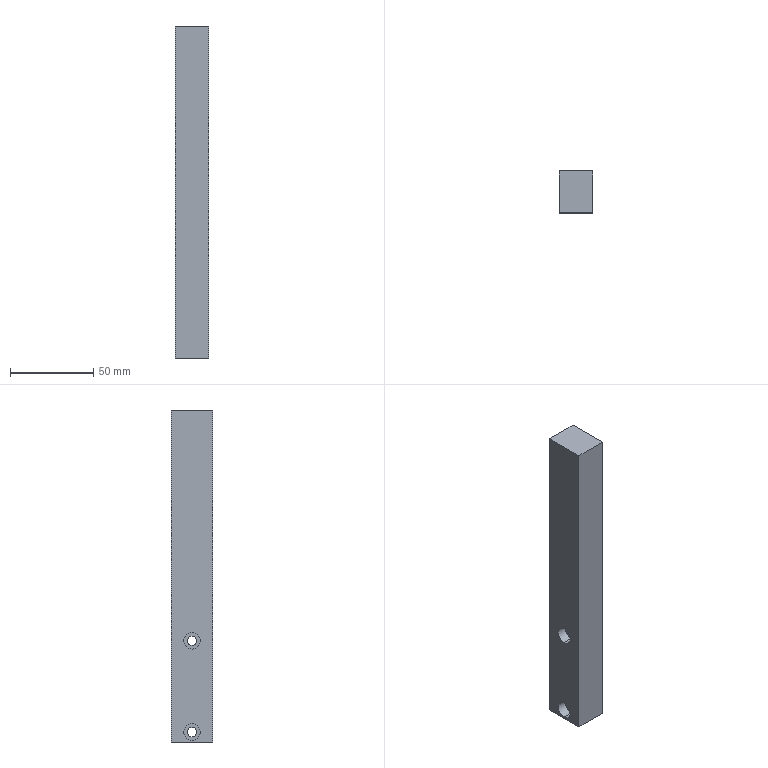Part | STEP file | PN_0058 push block | 1 solid | 16 faces | box 20 x 25 x 200 mm | volume 98425 mm3 | cylinder 8 | plane 8 | commonest cylinder face diameters 5.5 x4 10 x4
STEP:
#1=CARTESIAN_POINT('',(0.,0.,0.));
#2=DIRECTION('',(0.,0.,1.));
#3=DIRECTION('',(1.,0.,0.));
#4=AXIS2_PLACEMENT_3D('',#1,#2,#3);
#5=CARTESIAN_POINT('',(-4.3,0.,11.));
#6=VERTEX_POINT('',#5);
#7=CARTESIAN_POINT('',(-10.,0.,11.));
#8=VERTEX_POINT('',#7);
#9=CARTESIAN_POINT('',(-10.,0.,11.));
#10=DIRECTION('',(-1.,0.,0.));
#11=VECTOR('',#10,1.);
#12=LINE('',#9,#11);
#13=CARTESIAN_POINT('',(-10.,0.,6.));
#14=DIRECTION('',(-1.,0.,0.));
#15=DIRECTION('',(0.,0.,1.));
#16=AXIS2_PLACEMENT_3D('',#13,#14,#15);
#17=CYLINDRICAL_SURFACE('',#16,5.);
#18=CARTESIAN_POINT('',(6.283,0.));
#19=DIRECTION('',(0.,1.));
#20=VECTOR('',#19,1.);
#21=LINE('',#18,#20);
#22=(GEOMETRIC_REPRESENTATION_CONTEXT(2)PARAMETRIC_REPRESENTATION_CONTEXT()REPRESENTATION_CONTEXT('',''));
#23=DEFINITIONAL_REPRESENTATION('',(#21),#22);
#24=PCURVE('',#17,#23);
#25=CARTESIAN_POINT('',(-10.,0.,6.));
#26=DIRECTION('',(-1.,0.,0.));
#27=DIRECTION('',(0.,0.,1.));
#28=AXIS2_PLACEMENT_3D('',#25,#26,#27);
#29=CYLINDRICAL_SURFACE('',#28,5.);
#30=CARTESIAN_POINT('',(0.,0.));
#31=DIRECTION('',(0.,1.));
#32=VECTOR('',#31,1.);
#33=LINE('',#30,#32);
#34=(GEOMETRIC_REPRESENTATION_CONTEXT(2)PARAMETRIC_REPRESENTATION_CONTEXT()REPRESENTATION_CONTEXT('',''));
#35=DEFINITIONAL_REPRESENTATION('',(#33),#34);
#36=PCURVE('',#29,#35);
#37=SURFACE_CURVE('',#12,(#24,#36),.PCURVE_S1.);
#38=EDGE_CURVE('',#6,#8,#37,.T.);
#39=ORIENTED_EDGE('',*,*,#38,.T.);
#40=CARTESIAN_POINT('',(-10.,0.,1.));
#41=VERTEX_POINT('',#40);
#42=CARTESIAN_POINT('',(-10.,0.,6.));
#43=DIRECTION('',(-1.,0.,0.));
#44=DIRECTION('',(0.,0.,1.));
#45=AXIS2_PLACEMENT_3D('',#42,#43,#44);
#46=CIRCLE('',#45,5.);
#47=CARTESIAN_POINT('',(0.,0.));
#48=DIRECTION('',(1.,0.));
#49=VECTOR('',#48,1.);
#50=LINE('',#47,#49);
#51=(GEOMETRIC_REPRESENTATION_CONTEXT(2)PARAMETRIC_REPRESENTATION_CONTEXT()REPRESENTATION_CONTEXT('',''));
#52=DEFINITIONAL_REPRESENTATION('',(#50),#51);
#53=PCURVE('',#17,#52);
#54=CARTESIAN_POINT('',(-10.,12.5,0.));
#55=DIRECTION('',(1.,0.,0.));
#56=DIRECTION('',(0.,0.,-1.));
#57=AXIS2_PLACEMENT_3D('',#54,#55,#56);
#58=PLANE('',#57);
#59=CARTESIAN_POINT('',(-11.,-12.5));
#60=CARTESIAN_POINT('',(-11.,-3.84));
#61=CARTESIAN_POINT('',(-3.5,-8.17));
#62=CARTESIAN_POINT('',(4.,-12.5));
#63=CARTESIAN_POINT('',(-3.5,-16.83));
#64=CARTESIAN_POINT('',(-11.,-21.16));
#65=CARTESIAN_POINT('',(-11.,-12.5));
#66=(BOUNDED_CURVE()B_SPLINE_CURVE(2,(#59,#60,#61,#62,#63,#64,#65),.UNSPECIFIED.,.T.,.F.)B_SPLINE_CURVE_WITH_KNOTS((1,2,2,2,2,1),(-2.094,0.,2.094,4.189,6.283,8.378),.UNSPECIFIED.)CURVE()GEOMETRIC_REPRESENTATION_ITEM()RATIONAL_B_SPLINE_CURVE((1.,0.5,1.,0.5,1.,0.5,1.))REPRESENTATION_ITEM(''));
#67=(GEOMETRIC_REPRESENTATION_CONTEXT(2)PARAMETRIC_REPRESENTATION_CONTEXT()REPRESENTATION_CONTEXT('',''));
#68=DEFINITIONAL_REPRESENTATION('',(#66),#67);
#69=PCURVE('',#58,#68);
#70=SURFACE_CURVE('',#46,(#53,#69),.PCURVE_S1.);
#71=EDGE_CURVE('',#41,#8,#70,.T.);
#72=ORIENTED_EDGE('',*,*,#71,.F.);
#73=CARTESIAN_POINT('',(-4.3,0.,1.));
#74=VERTEX_POINT('',#73);
#75=CARTESIAN_POINT('',(-10.,0.,1.));
#76=DIRECTION('',(-1.,0.,0.));
#77=VECTOR('',#76,1.);
#78=LINE('',#75,#77);
#79=CARTESIAN_POINT('',(3.142,0.));
#80=DIRECTION('',(0.,1.));
#81=VECTOR('',#80,1.);
#82=LINE('',#79,#81);
#83=(GEOMETRIC_REPRESENTATION_CONTEXT(2)PARAMETRIC_REPRESENTATION_CONTEXT()REPRESENTATION_CONTEXT('',''));
#84=DEFINITIONAL_REPRESENTATION('',(#82),#83);
#85=PCURVE('',#17,#84);
#86=CARTESIAN_POINT('',(3.142,0.));
#87=DIRECTION('',(0.,1.));
#88=VECTOR('',#87,1.);
#89=LINE('',#86,#88);
#90=(GEOMETRIC_REPRESENTATION_CONTEXT(2)PARAMETRIC_REPRESENTATION_CONTEXT()REPRESENTATION_CONTEXT('',''));
#91=DEFINITIONAL_REPRESENTATION('',(#89),#90);
#92=PCURVE('',#29,#91);
#93=SURFACE_CURVE('',#78,(#85,#92),.PCURVE_S1.);
#94=EDGE_CURVE('',#74,#41,#93,.T.);
#95=ORIENTED_EDGE('',*,*,#94,.F.);
#96=CARTESIAN_POINT('',(-4.3,0.,6.));
#97=DIRECTION('',(-1.,0.,0.));
#98=DIRECTION('',(0.,0.,1.));
#99=AXIS2_PLACEMENT_3D('',#96,#97,#98);
#100=CIRCLE('',#99,5.);
#101=CARTESIAN_POINT('',(0.,-5.7));
#102=DIRECTION('',(1.,0.));
#103=VECTOR('',#102,1.);
#104=LINE('',#101,#103);
#105=(GEOMETRIC_REPRESENTATION_CONTEXT(2)PARAMETRIC_REPRESENTATION_CONTEXT()REPRESENTATION_CONTEXT('',''));
#106=DEFINITIONAL_REPRESENTATION('',(#104),#105);
#107=PCURVE('',#17,#106);
#108=CARTESIAN_POINT('',(-4.3,2.75,6.));
#109=DIRECTION('',(1.,0.,0.));
#110=DIRECTION('',(0.,0.,-1.));
#111=AXIS2_PLACEMENT_3D('',#108,#109,#110);
#112=PLANE('',#111);
#113=CARTESIAN_POINT('',(-5.,-2.75));
#114=CARTESIAN_POINT('',(-5.,5.91));
#115=CARTESIAN_POINT('',(2.5,1.58));
#116=CARTESIAN_POINT('',(10.,-2.75));
#117=CARTESIAN_POINT('',(2.5,-7.08));
#118=CARTESIAN_POINT('',(-5.,-11.41));
#119=CARTESIAN_POINT('',(-5.,-2.75));
#120=(BOUNDED_CURVE()B_SPLINE_CURVE(2,(#113,#114,#115,#116,#117,#118,#119),.UNSPECIFIED.,.T.,.F.)B_SPLINE_CURVE_WITH_KNOTS((1,2,2,2,2,1),(-2.094,0.,2.094,4.189,6.283,8.378),.UNSPECIFIED.)CURVE()GEOMETRIC_REPRESENTATION_ITEM()RATIONAL_B_SPLINE_CURVE((1.,0.5,1.,0.5,1.,0.5,1.))REPRESENTATION_ITEM(''));
#121=(GEOMETRIC_REPRESENTATION_CONTEXT(2)PARAMETRIC_REPRESENTATION_CONTEXT()REPRESENTATION_CONTEXT('',''));
#122=DEFINITIONAL_REPRESENTATION('',(#120),#121);
#123=PCURVE('',#112,#122);
#124=SURFACE_CURVE('',#100,(#107,#123),.PCURVE_S1.);
#125=EDGE_CURVE('',#74,#6,#124,.T.);
#126=ORIENTED_EDGE('',*,*,#125,.T.);
#127=EDGE_LOOP('',(#39,#72,#95,#126));
#128=FACE_BOUND('',#127,.F.);
#129=ADVANCED_FACE('',(#128),#17,.F.);
#130=CARTESIAN_POINT('',(10.,0.,8.75));
#131=VERTEX_POINT('',#130);
#132=CARTESIAN_POINT('',(-4.3,0.,8.75));
#133=VERTEX_POINT('',#132);
#134=CARTESIAN_POINT('',(-10.,0.,8.75));
#135=DIRECTION('',(-1.,0.,0.));
#136=VECTOR('',#135,1.);
#137=LINE('',#134,#136);
#138=CARTESIAN_POINT('',(-10.,0.,6.));
#139=DIRECTION('',(-1.,0.,0.));
#140=DIRECTION('',(0.,0.,1.));
#141=AXIS2_PLACEMENT_3D('',#138,#139,#140);
#142=CYLINDRICAL_SURFACE('',#141,2.75);
#143=CARTESIAN_POINT('',(6.283,0.));
#144=DIRECTION('',(0.,1.));
#145=VECTOR('',#144,1.);
#146=LINE('',#143,#145);
#147=(GEOMETRIC_REPRESENTATION_CONTEXT(2)PARAMETRIC_REPRESENTATION_CONTEXT()REPRESENTATION_CONTEXT('',''));
#148=DEFINITIONAL_REPRESENTATION('',(#146),#147);
#149=PCURVE('',#142,#148);
#150=CARTESIAN_POINT('',(-10.,0.,6.));
#151=DIRECTION('',(-1.,0.,0.));
#152=DIRECTION('',(0.,0.,1.));
#153=AXIS2_PLACEMENT_3D('',#150,#151,#152);
#154=CYLINDRICAL_SURFACE('',#153,2.75);
#155=CARTESIAN_POINT('',(0.,0.));
#156=DIRECTION('',(0.,1.));
#157=VECTOR('',#156,1.);
#158=LINE('',#155,#157);
#159=(GEOMETRIC_REPRESENTATION_CONTEXT(2)PARAMETRIC_REPRESENTATION_CONTEXT()REPRESENTATION_CONTEXT('',''));
#160=DEFINITIONAL_REPRESENTATION('',(#158),#159);
#161=PCURVE('',#154,#160);
#162=SURFACE_CURVE('',#137,(#149,#161),.PCURVE_S1.);
#163=EDGE_CURVE('',#131,#133,#162,.T.);
#164=ORIENTED_EDGE('',*,*,#163,.T.);
#165=CARTESIAN_POINT('',(-4.3,0.,3.25));
#166=VERTEX_POINT('',#165);
#167=CARTESIAN_POINT('',(-4.3,0.,6.));
#168=DIRECTION('',(-1.,0.,0.));
#169=DIRECTION('',(0.,0.,1.));
#170=AXIS2_PLACEMENT_3D('',#167,#168,#169);
#171=CIRCLE('',#170,2.75);
#172=CARTESIAN_POINT('',(0.,-5.7));
#173=DIRECTION('',(1.,0.));
#174=VECTOR('',#173,1.);
#175=LINE('',#172,#174);
#176=(GEOMETRIC_REPRESENTATION_CONTEXT(2)PARAMETRIC_REPRESENTATION_CONTEXT()REPRESENTATION_CONTEXT('',''));
#177=DEFINITIONAL_REPRESENTATION('',(#175),#176);
#178=PCURVE('',#142,#177);
#179=CARTESIAN_POINT('',(-2.75,-2.75));
#180=CARTESIAN_POINT('',(-2.75,2.013));
#181=CARTESIAN_POINT('',(1.375,-0.3684));
#182=CARTESIAN_POINT('',(5.5,-2.75));
#183=CARTESIAN_POINT('',(1.375,-5.132));
#184=CARTESIAN_POINT('',(-2.75,-7.513));
#185=CARTESIAN_POINT('',(-2.75,-2.75));
#186=(BOUNDED_CURVE()B_SPLINE_CURVE(2,(#179,#180,#181,#182,#183,#184,#185),.UNSPECIFIED.,.T.,.F.)B_SPLINE_CURVE_WITH_KNOTS((1,2,2,2,2,1),(-2.094,0.,2.094,4.189,6.283,8.378),.UNSPECIFIED.)CURVE()GEOMETRIC_REPRESENTATION_ITEM()RATIONAL_B_SPLINE_CURVE((1.,0.5,1.,0.5,1.,0.5,1.))REPRESENTATION_ITEM(''));
#187=(GEOMETRIC_REPRESENTATION_CONTEXT(2)PARAMETRIC_REPRESENTATION_CONTEXT()REPRESENTATION_CONTEXT('',''));
#188=DEFINITIONAL_REPRESENTATION('',(#186),#187);
#189=PCURVE('',#112,#188);
#190=SURFACE_CURVE('',#171,(#178,#189),.PCURVE_S1.);
#191=EDGE_CURVE('',#166,#133,#190,.T.);
#192=ORIENTED_EDGE('',*,*,#191,.F.);
#193=CARTESIAN_POINT('',(10.,0.,3.25));
#194=VERTEX_POINT('',#193);
#195=CARTESIAN_POINT('',(-10.,0.,3.25));
#196=DIRECTION('',(-1.,0.,0.));
#197=VECTOR('',#196,1.);
#198=LINE('',#195,#197);
#199=CARTESIAN_POINT('',(3.142,0.));
#200=DIRECTION('',(0.,1.));
#201=VECTOR('',#200,1.);
#202=LINE('',#199,#201);
#203=(GEOMETRIC_REPRESENTATION_CONTEXT(2)PARAMETRIC_REPRESENTATION_CONTEXT()REPRESENTATION_CONTEXT('',''));
#204=DEFINITIONAL_REPRESENTATION('',(#202),#203);
#205=PCURVE('',#142,#204);
#206=CARTESIAN_POINT('',(3.142,0.));
#207=DIRECTION('',(0.,1.));
#208=VECTOR('',#207,1.);
#209=LINE('',#206,#208);
#210=(GEOMETRIC_REPRESENTATION_CONTEXT(2)PARAMETRIC_REPRESENTATION_CONTEXT()REPRESENTATION_CONTEXT('',''));
#211=DEFINITIONAL_REPRESENTATION('',(#209),#210);
#212=PCURVE('',#154,#211);
#213=SURFACE_CURVE('',#198,(#205,#212),.PCURVE_S1.);
#214=EDGE_CURVE('',#194,#166,#213,.T.);
#215=ORIENTED_EDGE('',*,*,#214,.F.);
#216=CARTESIAN_POINT('',(10.,0.,6.));
#217=DIRECTION('',(-1.,0.,0.));
#218=DIRECTION('',(0.,0.,1.));
#219=AXIS2_PLACEMENT_3D('',#216,#217,#218);
#220=CIRCLE('',#219,2.75);
#221=CARTESIAN_POINT('',(0.,-20.));
#222=DIRECTION('',(1.,0.));
#223=VECTOR('',#222,1.);
#224=LINE('',#221,#223);
#225=(GEOMETRIC_REPRESENTATION_CONTEXT(2)PARAMETRIC_REPRESENTATION_CONTEXT()REPRESENTATION_CONTEXT('',''));
#226=DEFINITIONAL_REPRESENTATION('',(#224),#225);
#227=PCURVE('',#142,#226);
#228=CARTESIAN_POINT('',(10.,12.5,0.));
#229=DIRECTION('',(-1.,0.,0.));
#230=DIRECTION('',(0.,0.,1.));
#231=AXIS2_PLACEMENT_3D('',#228,#229,#230);
#232=PLANE('',#231);
#233=CARTESIAN_POINT('',(6.,-12.5));
#234=DIRECTION('',(1.,0.));
#235=AXIS2_PLACEMENT_2D('',#233,#234);
#236=CIRCLE('',#235,2.75);
#237=(GEOMETRIC_REPRESENTATION_CONTEXT(2)PARAMETRIC_REPRESENTATION_CONTEXT()REPRESENTATION_CONTEXT('',''));
#238=DEFINITIONAL_REPRESENTATION('',(#236),#237);
#239=PCURVE('',#232,#238);
#240=SURFACE_CURVE('',#220,(#227,#239),.PCURVE_S1.);
#241=EDGE_CURVE('',#194,#131,#240,.T.);
#242=ORIENTED_EDGE('',*,*,#241,.T.);
#243=EDGE_LOOP('',(#164,#192,#215,#242));
#244=FACE_BOUND('',#243,.F.);
#245=ADVANCED_FACE('',(#244),#142,.F.);
#246=CARTESIAN_POINT('',(-4.3,0.,66.));
#247=VERTEX_POINT('',#246);
#248=CARTESIAN_POINT('',(-10.,0.,66.));
#249=VERTEX_POINT('',#248);
#250=CARTESIAN_POINT('',(-10.,0.,66.));
#251=DIRECTION('',(-1.,0.,0.));
#252=VECTOR('',#251,1.);
#253=LINE('',#250,#252);
#254=CARTESIAN_POINT('',(-10.,0.,61.));
#255=DIRECTION('',(-1.,0.,0.));
#256=DIRECTION('',(0.,0.,1.));
#257=AXIS2_PLACEMENT_3D('',#254,#255,#256);
#258=CYLINDRICAL_SURFACE('',#257,5.);
#259=CARTESIAN_POINT('',(6.283,0.));
#260=DIRECTION('',(0.,1.));
#261=VECTOR('',#260,1.);
#262=LINE('',#259,#261);
#263=(GEOMETRIC_REPRESENTATION_CONTEXT(2)PARAMETRIC_REPRESENTATION_CONTEXT()REPRESENTATION_CONTEXT('',''));
#264=DEFINITIONAL_REPRESENTATION('',(#262),#263);
#265=PCURVE('',#258,#264);
#266=CARTESIAN_POINT('',(-10.,0.,61.));
#267=DIRECTION('',(-1.,0.,0.));
#268=DIRECTION('',(0.,0.,1.));
#269=AXIS2_PLACEMENT_3D('',#266,#267,#268);
#270=CYLINDRICAL_SURFACE('',#269,5.);
#271=CARTESIAN_POINT('',(0.,0.));
#272=DIRECTION('',(0.,1.));
#273=VECTOR('',#272,1.);
#274=LINE('',#271,#273);
#275=(GEOMETRIC_REPRESENTATION_CONTEXT(2)PARAMETRIC_REPRESENTATION_CONTEXT()REPRESENTATION_CONTEXT('',''));
#276=DEFINITIONAL_REPRESENTATION('',(#274),#275);
#277=PCURVE('',#270,#276);
#278=SURFACE_CURVE('',#253,(#265,#277),.PCURVE_S1.);
#279=EDGE_CURVE('',#247,#249,#278,.T.);
#280=ORIENTED_EDGE('',*,*,#279,.T.);
#281=CARTESIAN_POINT('',(-10.,0.,56.));
#282=VERTEX_POINT('',#281);
#283=CARTESIAN_POINT('',(-10.,0.,61.));
#284=DIRECTION('',(-1.,0.,0.));
#285=DIRECTION('',(0.,0.,1.));
#286=AXIS2_PLACEMENT_3D('',#283,#284,#285);
#287=CIRCLE('',#286,5.);
#288=CARTESIAN_POINT('',(0.,0.));
#289=DIRECTION('',(1.,0.));
#290=VECTOR('',#289,1.);
#291=LINE('',#288,#290);
#292=(GEOMETRIC_REPRESENTATION_CONTEXT(2)PARAMETRIC_REPRESENTATION_CONTEXT()REPRESENTATION_CONTEXT('',''));
#293=DEFINITIONAL_REPRESENTATION('',(#291),#292);
#294=PCURVE('',#258,#293);
#295=CARTESIAN_POINT('',(-66.,-12.5));
#296=CARTESIAN_POINT('',(-66.,-3.84));
#297=CARTESIAN_POINT('',(-58.5,-8.17));
#298=CARTESIAN_POINT('',(-51.,-12.5));
#299=CARTESIAN_POINT('',(-58.5,-16.83));
#300=CARTESIAN_POINT('',(-66.,-21.16));
#301=CARTESIAN_POINT('',(-66.,-12.5));
#302=(BOUNDED_CURVE()B_SPLINE_CURVE(2,(#295,#296,#297,#298,#299,#300,#301),.UNSPECIFIED.,.T.,.F.)B_SPLINE_CURVE_WITH_KNOTS((1,2,2,2,2,1),(-2.094,0.,2.094,4.189,6.283,8.378),.UNSPECIFIED.)CURVE()GEOMETRIC_REPRESENTATION_ITEM()RATIONAL_B_SPLINE_CURVE((1.,0.5,1.,0.5,1.,0.5,1.))REPRESENTATION_ITEM(''));
#303=(GEOMETRIC_REPRESENTATION_CONTEXT(2)PARAMETRIC_REPRESENTATION_CONTEXT()REPRESENTATION_CONTEXT('',''));
#304=DEFINITIONAL_REPRESENTATION('',(#302),#303);
#305=PCURVE('',#58,#304);
#306=SURFACE_CURVE('',#287,(#294,#305),.PCURVE_S1.);
#307=EDGE_CURVE('',#282,#249,#306,.T.);
#308=ORIENTED_EDGE('',*,*,#307,.F.);
#309=CARTESIAN_POINT('',(-4.3,0.,56.));
#310=VERTEX_POINT('',#309);
#311=CARTESIAN_POINT('',(-10.,0.,56.));
#312=DIRECTION('',(-1.,0.,0.));
#313=VECTOR('',#312,1.);
#314=LINE('',#311,#313);
#315=CARTESIAN_POINT('',(3.142,0.));
#316=DIRECTION('',(0.,1.));
#317=VECTOR('',#316,1.);
#318=LINE('',#315,#317);
#319=(GEOMETRIC_REPRESENTATION_CONTEXT(2)PARAMETRIC_REPRESENTATION_CONTEXT()REPRESENTATION_CONTEXT('',''));
#320=DEFINITIONAL_REPRESENTATION('',(#318),#319);
#321=PCURVE('',#258,#320);
#322=CARTESIAN_POINT('',(3.142,0.));
#323=DIRECTION('',(0.,1.));
#324=VECTOR('',#323,1.);
#325=LINE('',#322,#324);
#326=(GEOMETRIC_REPRESENTATION_CONTEXT(2)PARAMETRIC_REPRESENTATION_CONTEXT()REPRESENTATION_CONTEXT('',''));
#327=DEFINITIONAL_REPRESENTATION('',(#325),#326);
#328=PCURVE('',#270,#327);
#329=SURFACE_CURVE('',#314,(#321,#328),.PCURVE_S1.);
#330=EDGE_CURVE('',#310,#282,#329,.T.);
#331=ORIENTED_EDGE('',*,*,#330,.F.);
#332=CARTESIAN_POINT('',(-4.3,0.,61.));
#333=DIRECTION('',(-1.,0.,0.));
#334=DIRECTION('',(0.,0.,1.));
#335=AXIS2_PLACEMENT_3D('',#332,#333,#334);
#336=CIRCLE('',#335,5.);
#337=CARTESIAN_POINT('',(0.,-5.7));
#338=DIRECTION('',(1.,0.));
#339=VECTOR('',#338,1.);
#340=LINE('',#337,#339);
#341=(GEOMETRIC_REPRESENTATION_CONTEXT(2)PARAMETRIC_REPRESENTATION_CONTEXT()REPRESENTATION_CONTEXT('',''));
#342=DEFINITIONAL_REPRESENTATION('',(#340),#341);
#343=PCURVE('',#258,#342);
#344=CARTESIAN_POINT('',(-4.3,2.75,61.));
#345=DIRECTION('',(1.,0.,0.));
#346=DIRECTION('',(0.,0.,-1.));
#347=AXIS2_PLACEMENT_3D('',#344,#345,#346);
#348=PLANE('',#347);
#349=CARTESIAN_POINT('',(-5.,-2.75));
#350=CARTESIAN_POINT('',(-5.,5.91));
#351=CARTESIAN_POINT('',(2.5,1.58));
#352=CARTESIAN_POINT('',(10.,-2.75));
#353=CARTESIAN_POINT('',(2.5,-7.08));
#354=CARTESIAN_POINT('',(-5.,-11.41));
#355=CARTESIAN_POINT('',(-5.,-2.75));
#356=(BOUNDED_CURVE()B_SPLINE_CURVE(2,(#349,#350,#351,#352,#353,#354,#355),.UNSPECIFIED.,.T.,.F.)B_SPLINE_CURVE_WITH_KNOTS((1,2,2,2,2,1),(-2.094,0.,2.094,4.189,6.283,8.378),.UNSPECIFIED.)CURVE()GEOMETRIC_REPRESENTATION_ITEM()RATIONAL_B_SPLINE_CURVE((1.,0.5,1.,0.5,1.,0.5,1.))REPRESENTATION_ITEM(''));
#357=(GEOMETRIC_REPRESENTATION_CONTEXT(2)PARAMETRIC_REPRESENTATION_CONTEXT()REPRESENTATION_CONTEXT('',''));
#358=DEFINITIONAL_REPRESENTATION('',(#356),#357);
#359=PCURVE('',#348,#358);
#360=SURFACE_CURVE('',#336,(#343,#359),.PCURVE_S1.);
#361=EDGE_CURVE('',#310,#247,#360,.T.);
#362=ORIENTED_EDGE('',*,*,#361,.T.);
#363=EDGE_LOOP('',(#280,#308,#331,#362));
#364=FACE_BOUND('',#363,.F.);
#365=ADVANCED_FACE('',(#364),#258,.F.);
#366=CARTESIAN_POINT('',(10.,0.,63.75));
#367=VERTEX_POINT('',#366);
#368=CARTESIAN_POINT('',(-4.3,0.,63.75));
#369=VERTEX_POINT('',#368);
#370=CARTESIAN_POINT('',(-10.,0.,63.75));
#371=DIRECTION('',(-1.,0.,0.));
#372=VECTOR('',#371,1.);
#373=LINE('',#370,#372);
#374=CARTESIAN_POINT('',(-10.,0.,61.));
#375=DIRECTION('',(-1.,0.,0.));
#376=DIRECTION('',(0.,0.,1.));
#377=AXIS2_PLACEMENT_3D('',#374,#375,#376);
#378=CYLINDRICAL_SURFACE('',#377,2.75);
#379=CARTESIAN_POINT('',(6.283,0.));
#380=DIRECTION('',(0.,1.));
#381=VECTOR('',#380,1.);
#382=LINE('',#379,#381);
#383=(GEOMETRIC_REPRESENTATION_CONTEXT(2)PARAMETRIC_REPRESENTATION_CONTEXT()REPRESENTATION_CONTEXT('',''));
#384=DEFINITIONAL_REPRESENTATION('',(#382),#383);
#385=PCURVE('',#378,#384);
#386=CARTESIAN_POINT('',(-10.,0.,61.));
#387=DIRECTION('',(-1.,0.,0.));
#388=DIRECTION('',(0.,0.,1.));
#389=AXIS2_PLACEMENT_3D('',#386,#387,#388);
#390=CYLINDRICAL_SURFACE('',#389,2.75);
#391=CARTESIAN_POINT('',(0.,0.));
#392=DIRECTION('',(0.,1.));
#393=VECTOR('',#392,1.);
#394=LINE('',#391,#393);
#395=(GEOMETRIC_REPRESENTATION_CONTEXT(2)PARAMETRIC_REPRESENTATION_CONTEXT()REPRESENTATION_CONTEXT('',''));
#396=DEFINITIONAL_REPRESENTATION('',(#394),#395);
#397=PCURVE('',#390,#396);
#398=SURFACE_CURVE('',#373,(#385,#397),.PCURVE_S1.);
#399=EDGE_CURVE('',#367,#369,#398,.T.);
#400=ORIENTED_EDGE('',*,*,#399,.T.);
#401=CARTESIAN_POINT('',(-4.3,0.,58.25));
#402=VERTEX_POINT('',#401);
#403=CARTESIAN_POINT('',(-4.3,0.,61.));
#404=DIRECTION('',(-1.,0.,0.));
#405=DIRECTION('',(0.,0.,1.));
#406=AXIS2_PLACEMENT_3D('',#403,#404,#405);
#407=CIRCLE('',#406,2.75);
#408=CARTESIAN_POINT('',(0.,-5.7));
#409=DIRECTION('',(1.,0.));
#410=VECTOR('',#409,1.);
#411=LINE('',#408,#410);
#412=(GEOMETRIC_REPRESENTATION_CONTEXT(2)PARAMETRIC_REPRESENTATION_CONTEXT()REPRESENTATION_CONTEXT('',''));
#413=DEFINITIONAL_REPRESENTATION('',(#411),#412);
#414=PCURVE('',#378,#413);
#415=CARTESIAN_POINT('',(-2.75,-2.75));
#416=CARTESIAN_POINT('',(-2.75,2.013));
#417=CARTESIAN_POINT('',(1.375,-0.3684));
#418=CARTESIAN_POINT('',(5.5,-2.75));
#419=CARTESIAN_POINT('',(1.375,-5.132));
#420=CARTESIAN_POINT('',(-2.75,-7.513));
#421=CARTESIAN_POINT('',(-2.75,-2.75));
#422=(BOUNDED_CURVE()B_SPLINE_CURVE(2,(#415,#416,#417,#418,#419,#420,#421),.UNSPECIFIED.,.T.,.F.)B_SPLINE_CURVE_WITH_KNOTS((1,2,2,2,2,1),(-2.094,0.,2.094,4.189,6.283,8.378),.UNSPECIFIED.)CURVE()GEOMETRIC_REPRESENTATION_ITEM()RATIONAL_B_SPLINE_CURVE((1.,0.5,1.,0.5,1.,0.5,1.))REPRESENTATION_ITEM(''));
#423=(GEOMETRIC_REPRESENTATION_CONTEXT(2)PARAMETRIC_REPRESENTATION_CONTEXT()REPRESENTATION_CONTEXT('',''));
#424=DEFINITIONAL_REPRESENTATION('',(#422),#423);
#425=PCURVE('',#348,#424);
#426=SURFACE_CURVE('',#407,(#414,#425),.PCURVE_S1.);
#427=EDGE_CURVE('',#402,#369,#426,.T.);
#428=ORIENTED_EDGE('',*,*,#427,.F.);
#429=CARTESIAN_POINT('',(10.,0.,58.25));
#430=VERTEX_POINT('',#429);
#431=CARTESIAN_POINT('',(-10.,0.,58.25));
#432=DIRECTION('',(-1.,0.,0.));
#433=VECTOR('',#432,1.);
#434=LINE('',#431,#433);
#435=CARTESIAN_POINT('',(3.142,0.));
#436=DIRECTION('',(0.,1.));
#437=VECTOR('',#436,1.);
#438=LINE('',#435,#437);
#439=(GEOMETRIC_REPRESENTATION_CONTEXT(2)PARAMETRIC_REPRESENTATION_CONTEXT()REPRESENTATION_CONTEXT('',''));
#440=DEFINITIONAL_REPRESENTATION('',(#438),#439);
#441=PCURVE('',#378,#440);
#442=CARTESIAN_POINT('',(3.142,0.));
#443=DIRECTION('',(0.,1.));
#444=VECTOR('',#443,1.);
#445=LINE('',#442,#444);
#446=(GEOMETRIC_REPRESENTATION_CONTEXT(2)PARAMETRIC_REPRESENTATION_CONTEXT()REPRESENTATION_CONTEXT('',''));
#447=DEFINITIONAL_REPRESENTATION('',(#445),#446);
#448=PCURVE('',#390,#447);
#449=SURFACE_CURVE('',#434,(#441,#448),.PCURVE_S1.);
#450=EDGE_CURVE('',#430,#402,#449,.T.);
#451=ORIENTED_EDGE('',*,*,#450,.F.);
#452=CARTESIAN_POINT('',(10.,0.,61.));
#453=DIRECTION('',(-1.,0.,0.));
#454=DIRECTION('',(0.,0.,1.));
#455=AXIS2_PLACEMENT_3D('',#452,#453,#454);
#456=CIRCLE('',#455,2.75);
#457=CARTESIAN_POINT('',(0.,-20.));
#458=DIRECTION('',(1.,0.));
#459=VECTOR('',#458,1.);
#460=LINE('',#457,#459);
#461=(GEOMETRIC_REPRESENTATION_CONTEXT(2)PARAMETRIC_REPRESENTATION_CONTEXT()REPRESENTATION_CONTEXT('',''));
#462=DEFINITIONAL_REPRESENTATION('',(#460),#461);
#463=PCURVE('',#378,#462);
#464=CARTESIAN_POINT('',(61.,-12.5));
#465=DIRECTION('',(1.,0.));
#466=AXIS2_PLACEMENT_2D('',#464,#465);
#467=CIRCLE('',#466,2.75);
#468=(GEOMETRIC_REPRESENTATION_CONTEXT(2)PARAMETRIC_REPRESENTATION_CONTEXT()REPRESENTATION_CONTEXT('',''));
#469=DEFINITIONAL_REPRESENTATION('',(#467),#468);
#470=PCURVE('',#232,#469);
#471=SURFACE_CURVE('',#456,(#463,#470),.PCURVE_S1.);
#472=EDGE_CURVE('',#430,#367,#471,.T.);
#473=ORIENTED_EDGE('',*,*,#472,.T.);
#474=EDGE_LOOP('',(#400,#428,#451,#473));
#475=FACE_BOUND('',#474,.F.);
#476=ADVANCED_FACE('',(#475),#378,.F.);
#477=CARTESIAN_POINT('',(-10.,0.,6.));
#478=DIRECTION('',(-1.,0.,0.));
#479=DIRECTION('',(0.,0.,1.));
#480=AXIS2_PLACEMENT_3D('',#477,#478,#479);
#481=CIRCLE('',#480,5.);
#482=CARTESIAN_POINT('',(-11.,-12.5));
#483=CARTESIAN_POINT('',(-11.,-3.84));
#484=CARTESIAN_POINT('',(-3.5,-8.17));
#485=CARTESIAN_POINT('',(4.,-12.5));
#486=CARTESIAN_POINT('',(-3.5,-16.83));
#487=CARTESIAN_POINT('',(-11.,-21.16));
#488=CARTESIAN_POINT('',(-11.,-12.5));
#489=(BOUNDED_CURVE()B_SPLINE_CURVE(2,(#482,#483,#484,#485,#486,#487,#488),.UNSPECIFIED.,.T.,.F.)B_SPLINE_CURVE_WITH_KNOTS((1,2,2,2,2,1),(-2.094,0.,2.094,4.189,6.283,8.378),.UNSPECIFIED.)CURVE()GEOMETRIC_REPRESENTATION_ITEM()RATIONAL_B_SPLINE_CURVE((1.,0.5,1.,0.5,1.,0.5,1.))REPRESENTATION_ITEM(''));
#490=(GEOMETRIC_REPRESENTATION_CONTEXT(2)PARAMETRIC_REPRESENTATION_CONTEXT()REPRESENTATION_CONTEXT('',''));
#491=DEFINITIONAL_REPRESENTATION('',(#489),#490);
#492=PCURVE('',#58,#491);
#493=CARTESIAN_POINT('',(0.,0.));
#494=DIRECTION('',(1.,0.));
#495=VECTOR('',#494,1.);
#496=LINE('',#493,#495);
#497=(GEOMETRIC_REPRESENTATION_CONTEXT(2)PARAMETRIC_REPRESENTATION_CONTEXT()REPRESENTATION_CONTEXT('',''));
#498=DEFINITIONAL_REPRESENTATION('',(#496),#497);
#499=PCURVE('',#29,#498);
#500=SURFACE_CURVE('',#481,(#492,#499),.PCURVE_S1.);
#501=EDGE_CURVE('',#8,#41,#500,.T.);
#502=ORIENTED_EDGE('',*,*,#501,.F.);
#503=ORIENTED_EDGE('',*,*,#71,.F.);
#504=EDGE_LOOP('',(#502,#503));
#505=FACE_BOUND('',#504,.T.);
#506=CARTESIAN_POINT('',(-10.,0.,61.));
#507=DIRECTION('',(-1.,0.,0.));
#508=DIRECTION('',(0.,0.,1.));
#509=AXIS2_PLACEMENT_3D('',#506,#507,#508);
#510=CIRCLE('',#509,5.);
#511=CARTESIAN_POINT('',(-66.,-12.5));
#512=CARTESIAN_POINT('',(-66.,-3.84));
#513=CARTESIAN_POINT('',(-58.5,-8.17));
#514=CARTESIAN_POINT('',(-51.,-12.5));
#515=CARTESIAN_POINT('',(-58.5,-16.83));
#516=CARTESIAN_POINT('',(-66.,-21.16));
#517=CARTESIAN_POINT('',(-66.,-12.5));
#518=(BOUNDED_CURVE()B_SPLINE_CURVE(2,(#511,#512,#513,#514,#515,#516,#517),.UNSPECIFIED.,.T.,.F.)B_SPLINE_CURVE_WITH_KNOTS((1,2,2,2,2,1),(-2.094,0.,2.094,4.189,6.283,8.378),.UNSPECIFIED.)CURVE()GEOMETRIC_REPRESENTATION_ITEM()RATIONAL_B_SPLINE_CURVE((1.,0.5,1.,0.5,1.,0.5,1.))REPRESENTATION_ITEM(''));
#519=(GEOMETRIC_REPRESENTATION_CONTEXT(2)PARAMETRIC_REPRESENTATION_CONTEXT()REPRESENTATION_CONTEXT('',''));
#520=DEFINITIONAL_REPRESENTATION('',(#518),#519);
#521=PCURVE('',#58,#520);
#522=CARTESIAN_POINT('',(0.,0.));
#523=DIRECTION('',(1.,0.));
#524=VECTOR('',#523,1.);
#525=LINE('',#522,#524);
#526=(GEOMETRIC_REPRESENTATION_CONTEXT(2)PARAMETRIC_REPRESENTATION_CONTEXT()REPRESENTATION_CONTEXT('',''));
#527=DEFINITIONAL_REPRESENTATION('',(#525),#526);
#528=PCURVE('',#270,#527);
#529=SURFACE_CURVE('',#510,(#521,#528),.PCURVE_S1.);
#530=EDGE_CURVE('',#249,#282,#529,.T.);
#531=ORIENTED_EDGE('',*,*,#530,.F.);
#532=ORIENTED_EDGE('',*,*,#307,.F.);
#533=EDGE_LOOP('',(#531,#532));
#534=FACE_BOUND('',#533,.T.);
#535=CARTESIAN_POINT('',(-10.,-12.5,0.));
#536=VERTEX_POINT('',#535);
#537=CARTESIAN_POINT('',(-10.,-12.5,200.));
#538=VERTEX_POINT('',#537);
#539=CARTESIAN_POINT('',(-10.,-12.5,0.));
#540=DIRECTION('',(0.,0.,1.));
#541=VECTOR('',#540,1.);
#542=LINE('',#539,#541);
#543=CARTESIAN_POINT('',(0.,-25.));
#544=DIRECTION('',(-1.,0.));
#545=VECTOR('',#544,1.);
#546=LINE('',#543,#545);
#547=(GEOMETRIC_REPRESENTATION_CONTEXT(2)PARAMETRIC_REPRESENTATION_CONTEXT()REPRESENTATION_CONTEXT('',''));
#548=DEFINITIONAL_REPRESENTATION('',(#546),#547);
#549=PCURVE('',#58,#548);
#550=CARTESIAN_POINT('',(0.,-12.5,0.));
#551=DIRECTION('',(0.,1.,0.));
#552=DIRECTION('',(0.,0.,1.));
#553=AXIS2_PLACEMENT_3D('',#550,#551,#552);
#554=PLANE('',#553);
#555=CARTESIAN_POINT('',(0.,-10.));
#556=DIRECTION('',(1.,0.));
#557=VECTOR('',#556,1.);
#558=LINE('',#555,#557);
#559=(GEOMETRIC_REPRESENTATION_CONTEXT(2)PARAMETRIC_REPRESENTATION_CONTEXT()REPRESENTATION_CONTEXT('',''));
#560=DEFINITIONAL_REPRESENTATION('',(#558),#559);
#561=PCURVE('',#554,#560);
#562=SURFACE_CURVE('',#542,(#549,#561),.PCURVE_S1.);
#563=EDGE_CURVE('',#536,#538,#562,.T.);
#564=ORIENTED_EDGE('',*,*,#563,.T.);
#565=CARTESIAN_POINT('',(-10.,12.5,200.));
#566=VERTEX_POINT('',#565);
#567=CARTESIAN_POINT('',(-10.,12.5,200.));
#568=DIRECTION('',(0.,-1.,0.));
#569=VECTOR('',#568,1.);
#570=LINE('',#567,#569);
#571=CARTESIAN_POINT('',(-200.,0.));
#572=DIRECTION('',(0.,-1.));
#573=VECTOR('',#572,1.);
#574=LINE('',#571,#573);
#575=(GEOMETRIC_REPRESENTATION_CONTEXT(2)PARAMETRIC_REPRESENTATION_CONTEXT()REPRESENTATION_CONTEXT('',''));
#576=DEFINITIONAL_REPRESENTATION('',(#574),#575);
#577=PCURVE('',#58,#576);
#578=CARTESIAN_POINT('',(-10.,12.5,200.));
#579=DIRECTION('',(0.,0.,-1.));
#580=DIRECTION('',(-1.,0.,0.));
#581=AXIS2_PLACEMENT_3D('',#578,#579,#580);
#582=PLANE('',#581);
#583=CARTESIAN_POINT('',(0.,0.));
#584=DIRECTION('',(0.,-1.));
#585=VECTOR('',#584,1.);
#586=LINE('',#583,#585);
#587=(GEOMETRIC_REPRESENTATION_CONTEXT(2)PARAMETRIC_REPRESENTATION_CONTEXT()REPRESENTATION_CONTEXT('',''));
#588=DEFINITIONAL_REPRESENTATION('',(#586),#587);
#589=PCURVE('',#582,#588);
#590=SURFACE_CURVE('',#570,(#577,#589),.PCURVE_S1.);
#591=EDGE_CURVE('',#566,#538,#590,.T.);
#592=ORIENTED_EDGE('',*,*,#591,.F.);
#593=CARTESIAN_POINT('',(-10.,12.5,0.));
#594=VERTEX_POINT('',#593);
#595=CARTESIAN_POINT('',(-10.,12.5,0.));
#596=DIRECTION('',(0.,0.,1.));
#597=VECTOR('',#596,1.);
#598=LINE('',#595,#597);
#599=CARTESIAN_POINT('',(0.,0.));
#600=DIRECTION('',(-1.,0.));
#601=VECTOR('',#600,1.);
#602=LINE('',#599,#601);
#603=(GEOMETRIC_REPRESENTATION_CONTEXT(2)PARAMETRIC_REPRESENTATION_CONTEXT()REPRESENTATION_CONTEXT('',''));
#604=DEFINITIONAL_REPRESENTATION('',(#602),#603);
#605=PCURVE('',#58,#604);
#606=CARTESIAN_POINT('',(0.,12.5,0.));
#607=DIRECTION('',(0.,1.,0.));
#608=DIRECTION('',(0.,0.,1.));
#609=AXIS2_PLACEMENT_3D('',#606,#607,#608);
#610=PLANE('',#609);
#611=CARTESIAN_POINT('',(0.,-10.));
#612=DIRECTION('',(1.,0.));
#613=VECTOR('',#612,1.);
#614=LINE('',#611,#613);
#615=(GEOMETRIC_REPRESENTATION_CONTEXT(2)PARAMETRIC_REPRESENTATION_CONTEXT()REPRESENTATION_CONTEXT('',''));
#616=DEFINITIONAL_REPRESENTATION('',(#614),#615);
#617=PCURVE('',#610,#616);
#618=SURFACE_CURVE('',#598,(#605,#617),.PCURVE_S1.);
#619=EDGE_CURVE('',#594,#566,#618,.T.);
#620=ORIENTED_EDGE('',*,*,#619,.F.);
#621=CARTESIAN_POINT('',(-10.,12.5,0.));
#622=DIRECTION('',(0.,-1.,0.));
#623=VECTOR('',#622,1.);
#624=LINE('',#621,#623);
#625=CARTESIAN_POINT('',(0.,0.));
#626=DIRECTION('',(0.,-1.));
#627=VECTOR('',#626,1.);
#628=LINE('',#625,#627);
#629=(GEOMETRIC_REPRESENTATION_CONTEXT(2)PARAMETRIC_REPRESENTATION_CONTEXT()REPRESENTATION_CONTEXT('',''));
#630=DEFINITIONAL_REPRESENTATION('',(#628),#629);
#631=PCURVE('',#58,#630);
#632=CARTESIAN_POINT('',(-10.,12.5,0.));
#633=DIRECTION('',(0.,0.,1.));
#634=DIRECTION('',(1.,0.,0.));
#635=AXIS2_PLACEMENT_3D('',#632,#633,#634);
#636=PLANE('',#635);
#637=CARTESIAN_POINT('',(0.,0.));
#638=DIRECTION('',(0.,-1.));
#639=VECTOR('',#638,1.);
#640=LINE('',#637,#639);
#641=(GEOMETRIC_REPRESENTATION_CONTEXT(2)PARAMETRIC_REPRESENTATION_CONTEXT()REPRESENTATION_CONTEXT('',''));
#642=DEFINITIONAL_REPRESENTATION('',(#640),#641);
#643=PCURVE('',#636,#642);
#644=SURFACE_CURVE('',#624,(#631,#643),.PCURVE_S1.);
#645=EDGE_CURVE('',#594,#536,#644,.T.);
#646=ORIENTED_EDGE('',*,*,#645,.T.);
#647=EDGE_LOOP('',(#564,#592,#620,#646));
#648=FACE_BOUND('',#647,.T.);
#649=ADVANCED_FACE('',(#505,#534,#648),#58,.F.);
#650=CARTESIAN_POINT('',(10.,-12.5,200.));
#651=VERTEX_POINT('',#650);
#652=CARTESIAN_POINT('',(-10.,-12.5,200.));
#653=DIRECTION('',(1.,0.,0.));
#654=VECTOR('',#653,1.);
#655=LINE('',#652,#654);
#656=CARTESIAN_POINT('',(0.,-25.));
#657=DIRECTION('',(-1.,0.));
#658=VECTOR('',#657,1.);
#659=LINE('',#656,#658);
#660=(GEOMETRIC_REPRESENTATION_CONTEXT(2)PARAMETRIC_REPRESENTATION_CONTEXT()REPRESENTATION_CONTEXT('',''));
#661=DEFINITIONAL_REPRESENTATION('',(#659),#660);
#662=PCURVE('',#582,#661);
#663=CARTESIAN_POINT('',(200.,-10.));
#664=DIRECTION('',(0.,1.));
#665=VECTOR('',#664,1.);
#666=LINE('',#663,#665);
#667=(GEOMETRIC_REPRESENTATION_CONTEXT(2)PARAMETRIC_REPRESENTATION_CONTEXT()REPRESENTATION_CONTEXT('',''));
#668=DEFINITIONAL_REPRESENTATION('',(#666),#667);
#669=PCURVE('',#554,#668);
#670=SURFACE_CURVE('',#655,(#662,#669),.PCURVE_S1.);
#671=EDGE_CURVE('',#538,#651,#670,.T.);
#672=ORIENTED_EDGE('',*,*,#671,.T.);
#673=CARTESIAN_POINT('',(10.,12.5,200.));
#674=VERTEX_POINT('',#673);
#675=CARTESIAN_POINT('',(10.,12.5,200.));
#676=DIRECTION('',(0.,-1.,0.));
#677=VECTOR('',#676,1.);
#678=LINE('',#675,#677);
#679=CARTESIAN_POINT('',(-20.,0.));
#680=DIRECTION('',(0.,-1.));
#681=VECTOR('',#680,1.);
#682=LINE('',#679,#681);
#683=(GEOMETRIC_REPRESENTATION_CONTEXT(2)PARAMETRIC_REPRESENTATION_CONTEXT()REPRESENTATION_CONTEXT('',''));
#684=DEFINITIONAL_REPRESENTATION('',(#682),#683);
#685=PCURVE('',#582,#684);
#686=CARTESIAN_POINT('',(200.,0.));
#687=DIRECTION('',(0.,-1.));
#688=VECTOR('',#687,1.);
#689=LINE('',#686,#688);
#690=(GEOMETRIC_REPRESENTATION_CONTEXT(2)PARAMETRIC_REPRESENTATION_CONTEXT()REPRESENTATION_CONTEXT('',''));
#691=DEFINITIONAL_REPRESENTATION('',(#689),#690);
#692=PCURVE('',#232,#691);
#693=SURFACE_CURVE('',#678,(#685,#692),.PCURVE_S1.);
#694=EDGE_CURVE('',#674,#651,#693,.T.);
#695=ORIENTED_EDGE('',*,*,#694,.F.);
#696=CARTESIAN_POINT('',(-10.,12.5,200.));
#697=DIRECTION('',(1.,0.,0.));
#698=VECTOR('',#697,1.);
#699=LINE('',#696,#698);
#700=CARTESIAN_POINT('',(0.,0.));
#701=DIRECTION('',(-1.,0.));
#702=VECTOR('',#701,1.);
#703=LINE('',#700,#702);
#704=(GEOMETRIC_REPRESENTATION_CONTEXT(2)PARAMETRIC_REPRESENTATION_CONTEXT()REPRESENTATION_CONTEXT('',''));
#705=DEFINITIONAL_REPRESENTATION('',(#703),#704);
#706=PCURVE('',#582,#705);
#707=CARTESIAN_POINT('',(200.,-10.));
#708=DIRECTION('',(0.,1.));
#709=VECTOR('',#708,1.);
#710=LINE('',#707,#709);
#711=(GEOMETRIC_REPRESENTATION_CONTEXT(2)PARAMETRIC_REPRESENTATION_CONTEXT()REPRESENTATION_CONTEXT('',''));
#712=DEFINITIONAL_REPRESENTATION('',(#710),#711);
#713=PCURVE('',#610,#712);
#714=SURFACE_CURVE('',#699,(#706,#713),.PCURVE_S1.);
#715=EDGE_CURVE('',#566,#674,#714,.T.);
#716=ORIENTED_EDGE('',*,*,#715,.F.);
#717=ORIENTED_EDGE('',*,*,#591,.T.);
#718=EDGE_LOOP('',(#672,#695,#716,#717));
#719=FACE_BOUND('',#718,.T.);
#720=ADVANCED_FACE('',(#719),#582,.F.);
#721=CARTESIAN_POINT('',(10.,0.,6.));
#722=DIRECTION('',(-1.,0.,0.));
#723=DIRECTION('',(0.,0.,1.));
#724=AXIS2_PLACEMENT_3D('',#721,#722,#723);
#725=CIRCLE('',#724,2.75);
#726=CARTESIAN_POINT('',(6.,-12.5));
#727=DIRECTION('',(1.,0.));
#728=AXIS2_PLACEMENT_2D('',#726,#727);
#729=CIRCLE('',#728,2.75);
#730=(GEOMETRIC_REPRESENTATION_CONTEXT(2)PARAMETRIC_REPRESENTATION_CONTEXT()REPRESENTATION_CONTEXT('',''));
#731=DEFINITIONAL_REPRESENTATION('',(#729),#730);
#732=PCURVE('',#232,#731);
#733=CARTESIAN_POINT('',(0.,-20.));
#734=DIRECTION('',(1.,0.));
#735=VECTOR('',#734,1.);
#736=LINE('',#733,#735);
#737=(GEOMETRIC_REPRESENTATION_CONTEXT(2)PARAMETRIC_REPRESENTATION_CONTEXT()REPRESENTATION_CONTEXT('',''));
#738=DEFINITIONAL_REPRESENTATION('',(#736),#737);
#739=PCURVE('',#154,#738);
#740=SURFACE_CURVE('',#725,(#732,#739),.PCURVE_S1.);
#741=EDGE_CURVE('',#131,#194,#740,.T.);
#742=ORIENTED_EDGE('',*,*,#741,.T.);
#743=ORIENTED_EDGE('',*,*,#241,.T.);
#744=EDGE_LOOP('',(#742,#743));
#745=FACE_BOUND('',#744,.T.);
#746=CARTESIAN_POINT('',(10.,0.,61.));
#747=DIRECTION('',(-1.,0.,0.));
#748=DIRECTION('',(0.,0.,1.));
#749=AXIS2_PLACEMENT_3D('',#746,#747,#748);
#750=CIRCLE('',#749,2.75);
#751=CARTESIAN_POINT('',(61.,-12.5));
#752=DIRECTION('',(1.,0.));
#753=AXIS2_PLACEMENT_2D('',#751,#752);
#754=CIRCLE('',#753,2.75);
#755=(GEOMETRIC_REPRESENTATION_CONTEXT(2)PARAMETRIC_REPRESENTATION_CONTEXT()REPRESENTATION_CONTEXT('',''));
#756=DEFINITIONAL_REPRESENTATION('',(#754),#755);
#757=PCURVE('',#232,#756);
#758=CARTESIAN_POINT('',(0.,-20.));
#759=DIRECTION('',(1.,0.));
#760=VECTOR('',#759,1.);
#761=LINE('',#758,#760);
#762=(GEOMETRIC_REPRESENTATION_CONTEXT(2)PARAMETRIC_REPRESENTATION_CONTEXT()REPRESENTATION_CONTEXT('',''));
#763=DEFINITIONAL_REPRESENTATION('',(#761),#762);
#764=PCURVE('',#390,#763);
#765=SURFACE_CURVE('',#750,(#757,#764),.PCURVE_S1.);
#766=EDGE_CURVE('',#367,#430,#765,.T.);
#767=ORIENTED_EDGE('',*,*,#766,.T.);
#768=ORIENTED_EDGE('',*,*,#472,.T.);
#769=EDGE_LOOP('',(#767,#768));
#770=FACE_BOUND('',#769,.T.);
#771=CARTESIAN_POINT('',(10.,-12.5,0.));
#772=VERTEX_POINT('',#771);
#773=CARTESIAN_POINT('',(10.,-12.5,0.));
#774=DIRECTION('',(0.,0.,-1.));
#775=VECTOR('',#774,1.);
#776=LINE('',#773,#775);
#777=CARTESIAN_POINT('',(0.,-25.));
#778=DIRECTION('',(-1.,0.));
#779=VECTOR('',#778,1.);
#780=LINE('',#777,#779);
#781=(GEOMETRIC_REPRESENTATION_CONTEXT(2)PARAMETRIC_REPRESENTATION_CONTEXT()REPRESENTATION_CONTEXT('',''));
#782=DEFINITIONAL_REPRESENTATION('',(#780),#781);
#783=PCURVE('',#232,#782);
#784=CARTESIAN_POINT('',(0.,10.));
#785=DIRECTION('',(-1.,0.));
#786=VECTOR('',#785,1.);
#787=LINE('',#784,#786);
#788=(GEOMETRIC_REPRESENTATION_CONTEXT(2)PARAMETRIC_REPRESENTATION_CONTEXT()REPRESENTATION_CONTEXT('',''));
#789=DEFINITIONAL_REPRESENTATION('',(#787),#788);
#790=PCURVE('',#554,#789);
#791=SURFACE_CURVE('',#776,(#783,#790),.PCURVE_S1.);
#792=EDGE_CURVE('',#651,#772,#791,.T.);
#793=ORIENTED_EDGE('',*,*,#792,.T.);
#794=CARTESIAN_POINT('',(10.,12.5,0.));
#795=VERTEX_POINT('',#794);
#796=CARTESIAN_POINT('',(10.,12.5,0.));
#797=DIRECTION('',(0.,-1.,0.));
#798=VECTOR('',#797,1.);
#799=LINE('',#796,#798);
#800=CARTESIAN_POINT('',(0.,0.));
#801=DIRECTION('',(0.,-1.));
#802=VECTOR('',#801,1.);
#803=LINE('',#800,#802);
#804=(GEOMETRIC_REPRESENTATION_CONTEXT(2)PARAMETRIC_REPRESENTATION_CONTEXT()REPRESENTATION_CONTEXT('',''));
#805=DEFINITIONAL_REPRESENTATION('',(#803),#804);
#806=PCURVE('',#232,#805);
#807=CARTESIAN_POINT('',(20.,0.));
#808=DIRECTION('',(0.,-1.));
#809=VECTOR('',#808,1.);
#810=LINE('',#807,#809);
#811=(GEOMETRIC_REPRESENTATION_CONTEXT(2)PARAMETRIC_REPRESENTATION_CONTEXT()REPRESENTATION_CONTEXT('',''));
#812=DEFINITIONAL_REPRESENTATION('',(#810),#811);
#813=PCURVE('',#636,#812);
#814=SURFACE_CURVE('',#799,(#806,#813),.PCURVE_S1.);
#815=EDGE_CURVE('',#795,#772,#814,.T.);
#816=ORIENTED_EDGE('',*,*,#815,.F.);
#817=CARTESIAN_POINT('',(10.,12.5,0.));
#818=DIRECTION('',(0.,0.,-1.));
#819=VECTOR('',#818,1.);
#820=LINE('',#817,#819);
#821=CARTESIAN_POINT('',(0.,0.));
#822=DIRECTION('',(-1.,0.));
#823=VECTOR('',#822,1.);
#824=LINE('',#821,#823);
#825=(GEOMETRIC_REPRESENTATION_CONTEXT(2)PARAMETRIC_REPRESENTATION_CONTEXT()REPRESENTATION_CONTEXT('',''));
#826=DEFINITIONAL_REPRESENTATION('',(#824),#825);
#827=PCURVE('',#232,#826);
#828=CARTESIAN_POINT('',(0.,10.));
#829=DIRECTION('',(-1.,0.));
#830=VECTOR('',#829,1.);
#831=LINE('',#828,#830);
#832=(GEOMETRIC_REPRESENTATION_CONTEXT(2)PARAMETRIC_REPRESENTATION_CONTEXT()REPRESENTATION_CONTEXT('',''));
#833=DEFINITIONAL_REPRESENTATION('',(#831),#832);
#834=PCURVE('',#610,#833);
#835=SURFACE_CURVE('',#820,(#827,#834),.PCURVE_S1.);
#836=EDGE_CURVE('',#674,#795,#835,.T.);
#837=ORIENTED_EDGE('',*,*,#836,.F.);
#838=ORIENTED_EDGE('',*,*,#694,.T.);
#839=EDGE_LOOP('',(#793,#816,#837,#838));
#840=FACE_BOUND('',#839,.T.);
#841=ADVANCED_FACE('',(#745,#770,#840),#232,.F.);
#842=CARTESIAN_POINT('',(-10.,-12.5,0.));
#843=DIRECTION('',(-1.,0.,0.));
#844=VECTOR('',#843,1.);
#845=LINE('',#842,#844);
#846=CARTESIAN_POINT('',(0.,-25.));
#847=DIRECTION('',(-1.,0.));
#848=VECTOR('',#847,1.);
#849=LINE('',#846,#848);
#850=(GEOMETRIC_REPRESENTATION_CONTEXT(2)PARAMETRIC_REPRESENTATION_CONTEXT()REPRESENTATION_CONTEXT('',''));
#851=DEFINITIONAL_REPRESENTATION('',(#849),#850);
#852=PCURVE('',#636,#851);
#853=CARTESIAN_POINT('',(0.,-10.));
#854=DIRECTION('',(0.,-1.));
#855=VECTOR('',#854,1.);
#856=LINE('',#853,#855);
#857=(GEOMETRIC_REPRESENTATION_CONTEXT(2)PARAMETRIC_REPRESENTATION_CONTEXT()REPRESENTATION_CONTEXT('',''));
#858=DEFINITIONAL_REPRESENTATION('',(#856),#857);
#859=PCURVE('',#554,#858);
#860=SURFACE_CURVE('',#845,(#852,#859),.PCURVE_S1.);
#861=EDGE_CURVE('',#772,#536,#860,.T.);
#862=ORIENTED_EDGE('',*,*,#861,.T.);
#863=ORIENTED_EDGE('',*,*,#645,.F.);
#864=CARTESIAN_POINT('',(-10.,12.5,0.));
#865=DIRECTION('',(-1.,0.,0.));
#866=VECTOR('',#865,1.);
#867=LINE('',#864,#866);
#868=CARTESIAN_POINT('',(0.,0.));
#869=DIRECTION('',(-1.,0.));
#870=VECTOR('',#869,1.);
#871=LINE('',#868,#870);
#872=(GEOMETRIC_REPRESENTATION_CONTEXT(2)PARAMETRIC_REPRESENTATION_CONTEXT()REPRESENTATION_CONTEXT('',''));
#873=DEFINITIONAL_REPRESENTATION('',(#871),#872);
#874=PCURVE('',#636,#873);
#875=CARTESIAN_POINT('',(0.,-10.));
#876=DIRECTION('',(0.,-1.));
#877=VECTOR('',#876,1.);
#878=LINE('',#875,#877);
#879=(GEOMETRIC_REPRESENTATION_CONTEXT(2)PARAMETRIC_REPRESENTATION_CONTEXT()REPRESENTATION_CONTEXT('',''));
#880=DEFINITIONAL_REPRESENTATION('',(#878),#879);
#881=PCURVE('',#610,#880);
#882=SURFACE_CURVE('',#867,(#874,#881),.PCURVE_S1.);
#883=EDGE_CURVE('',#795,#594,#882,.T.);
#884=ORIENTED_EDGE('',*,*,#883,.F.);
#885=ORIENTED_EDGE('',*,*,#815,.T.);
#886=EDGE_LOOP('',(#862,#863,#884,#885));
#887=FACE_BOUND('',#886,.T.);
#888=ADVANCED_FACE('',(#887),#636,.F.);
#889=ORIENTED_EDGE('',*,*,#619,.T.);
#890=ORIENTED_EDGE('',*,*,#715,.T.);
#891=ORIENTED_EDGE('',*,*,#836,.T.);
#892=ORIENTED_EDGE('',*,*,#883,.T.);
#893=EDGE_LOOP('',(#889,#890,#891,#892));
#894=FACE_BOUND('',#893,.T.);
#895=ADVANCED_FACE('',(#894),#610,.T.);
#896=ORIENTED_EDGE('',*,*,#563,.F.);
#897=ORIENTED_EDGE('',*,*,#861,.F.);
#898=ORIENTED_EDGE('',*,*,#792,.F.);
#899=ORIENTED_EDGE('',*,*,#671,.F.);
#900=EDGE_LOOP('',(#896,#897,#898,#899));
#901=FACE_BOUND('',#900,.T.);
#902=ADVANCED_FACE('',(#901),#554,.F.);
#903=CARTESIAN_POINT('',(-4.3,0.,61.));
#904=DIRECTION('',(-1.,0.,0.));
#905=DIRECTION('',(0.,0.,1.));
#906=AXIS2_PLACEMENT_3D('',#903,#904,#905);
#907=CIRCLE('',#906,2.75);
#908=CARTESIAN_POINT('',(0.,-5.7));
#909=DIRECTION('',(1.,0.));
#910=VECTOR('',#909,1.);
#911=LINE('',#908,#910);
#912=(GEOMETRIC_REPRESENTATION_CONTEXT(2)PARAMETRIC_REPRESENTATION_CONTEXT()REPRESENTATION_CONTEXT('',''));
#913=DEFINITIONAL_REPRESENTATION('',(#911),#912);
#914=PCURVE('',#390,#913);
#915=CARTESIAN_POINT('',(-2.75,-2.75));
#916=CARTESIAN_POINT('',(-2.75,2.013));
#917=CARTESIAN_POINT('',(1.375,-0.3684));
#918=CARTESIAN_POINT('',(5.5,-2.75));
#919=CARTESIAN_POINT('',(1.375,-5.132));
#920=CARTESIAN_POINT('',(-2.75,-7.513));
#921=CARTESIAN_POINT('',(-2.75,-2.75));
#922=(BOUNDED_CURVE()B_SPLINE_CURVE(2,(#915,#916,#917,#918,#919,#920,#921),.UNSPECIFIED.,.T.,.F.)B_SPLINE_CURVE_WITH_KNOTS((1,2,2,2,2,1),(-2.094,0.,2.094,4.189,6.283,8.378),.UNSPECIFIED.)CURVE()GEOMETRIC_REPRESENTATION_ITEM()RATIONAL_B_SPLINE_CURVE((1.,0.5,1.,0.5,1.,0.5,1.))REPRESENTATION_ITEM(''));
#923=(GEOMETRIC_REPRESENTATION_CONTEXT(2)PARAMETRIC_REPRESENTATION_CONTEXT()REPRESENTATION_CONTEXT('',''));
#924=DEFINITIONAL_REPRESENTATION('',(#922),#923);
#925=PCURVE('',#348,#924);
#926=SURFACE_CURVE('',#907,(#914,#925),.PCURVE_S1.);
#927=EDGE_CURVE('',#369,#402,#926,.T.);
#928=ORIENTED_EDGE('',*,*,#927,.F.);
#929=ORIENTED_EDGE('',*,*,#399,.F.);
#930=ORIENTED_EDGE('',*,*,#766,.T.);
#931=ORIENTED_EDGE('',*,*,#450,.T.);
#932=EDGE_LOOP('',(#928,#929,#930,#931));
#933=FACE_BOUND('',#932,.F.);
#934=ADVANCED_FACE('',(#933),#390,.F.);
#935=ORIENTED_EDGE('',*,*,#927,.F.);
#936=ORIENTED_EDGE('',*,*,#427,.F.);
#937=EDGE_LOOP('',(#935,#936));
#938=FACE_BOUND('',#937,.T.);
#939=CARTESIAN_POINT('',(-4.3,0.,61.));
#940=DIRECTION('',(-1.,0.,0.));
#941=DIRECTION('',(0.,0.,1.));
#942=AXIS2_PLACEMENT_3D('',#939,#940,#941);
#943=CIRCLE('',#942,5.);
#944=CARTESIAN_POINT('',(-5.,-2.75));
#945=CARTESIAN_POINT('',(-5.,5.91));
#946=CARTESIAN_POINT('',(2.5,1.58));
#947=CARTESIAN_POINT('',(10.,-2.75));
#948=CARTESIAN_POINT('',(2.5,-7.08));
#949=CARTESIAN_POINT('',(-5.,-11.41));
#950=CARTESIAN_POINT('',(-5.,-2.75));
#951=(BOUNDED_CURVE()B_SPLINE_CURVE(2,(#944,#945,#946,#947,#948,#949,#950),.UNSPECIFIED.,.T.,.F.)B_SPLINE_CURVE_WITH_KNOTS((1,2,2,2,2,1),(-2.094,0.,2.094,4.189,6.283,8.378),.UNSPECIFIED.)CURVE()GEOMETRIC_REPRESENTATION_ITEM()RATIONAL_B_SPLINE_CURVE((1.,0.5,1.,0.5,1.,0.5,1.))REPRESENTATION_ITEM(''));
#952=(GEOMETRIC_REPRESENTATION_CONTEXT(2)PARAMETRIC_REPRESENTATION_CONTEXT()REPRESENTATION_CONTEXT('',''));
#953=DEFINITIONAL_REPRESENTATION('',(#951),#952);
#954=PCURVE('',#348,#953);
#955=CARTESIAN_POINT('',(0.,-5.7));
#956=DIRECTION('',(1.,0.));
#957=VECTOR('',#956,1.);
#958=LINE('',#955,#957);
#959=(GEOMETRIC_REPRESENTATION_CONTEXT(2)PARAMETRIC_REPRESENTATION_CONTEXT()REPRESENTATION_CONTEXT('',''));
#960=DEFINITIONAL_REPRESENTATION('',(#958),#959);
#961=PCURVE('',#270,#960);
#962=SURFACE_CURVE('',#943,(#954,#961),.PCURVE_S1.);
#963=EDGE_CURVE('',#247,#310,#962,.T.);
#964=ORIENTED_EDGE('',*,*,#963,.T.);
#965=ORIENTED_EDGE('',*,*,#361,.T.);
#966=EDGE_LOOP('',(#964,#965));
#967=FACE_BOUND('',#966,.T.);
#968=ADVANCED_FACE('',(#938,#967),#348,.F.);
#969=ORIENTED_EDGE('',*,*,#530,.F.);
#970=ORIENTED_EDGE('',*,*,#279,.F.);
#971=ORIENTED_EDGE('',*,*,#963,.T.);
#972=ORIENTED_EDGE('',*,*,#330,.T.);
#973=EDGE_LOOP('',(#969,#970,#971,#972));
#974=FACE_BOUND('',#973,.F.);
#975=ADVANCED_FACE('',(#974),#270,.F.);
#976=CARTESIAN_POINT('',(-4.3,0.,6.));
#977=DIRECTION('',(-1.,0.,0.));
#978=DIRECTION('',(0.,0.,1.));
#979=AXIS2_PLACEMENT_3D('',#976,#977,#978);
#980=CIRCLE('',#979,2.75);
#981=CARTESIAN_POINT('',(0.,-5.7));
#982=DIRECTION('',(1.,0.));
#983=VECTOR('',#982,1.);
#984=LINE('',#981,#983);
#985=(GEOMETRIC_REPRESENTATION_CONTEXT(2)PARAMETRIC_REPRESENTATION_CONTEXT()REPRESENTATION_CONTEXT('',''));
#986=DEFINITIONAL_REPRESENTATION('',(#984),#985);
#987=PCURVE('',#154,#986);
#988=CARTESIAN_POINT('',(-2.75,-2.75));
#989=CARTESIAN_POINT('',(-2.75,2.013));
#990=CARTESIAN_POINT('',(1.375,-0.3684));
#991=CARTESIAN_POINT('',(5.5,-2.75));
#992=CARTESIAN_POINT('',(1.375,-5.132));
#993=CARTESIAN_POINT('',(-2.75,-7.513));
#994=CARTESIAN_POINT('',(-2.75,-2.75));
#995=(BOUNDED_CURVE()B_SPLINE_CURVE(2,(#988,#989,#990,#991,#992,#993,#994),.UNSPECIFIED.,.T.,.F.)B_SPLINE_CURVE_WITH_KNOTS((1,2,2,2,2,1),(-2.094,0.,2.094,4.189,6.283,8.378),.UNSPECIFIED.)CURVE()GEOMETRIC_REPRESENTATION_ITEM()RATIONAL_B_SPLINE_CURVE((1.,0.5,1.,0.5,1.,0.5,1.))REPRESENTATION_ITEM(''));
#996=(GEOMETRIC_REPRESENTATION_CONTEXT(2)PARAMETRIC_REPRESENTATION_CONTEXT()REPRESENTATION_CONTEXT('',''));
#997=DEFINITIONAL_REPRESENTATION('',(#995),#996);
#998=PCURVE('',#112,#997);
#999=SURFACE_CURVE('',#980,(#987,#998),.PCURVE_S1.);
#1000=EDGE_CURVE('',#133,#166,#999,.T.);
#1001=ORIENTED_EDGE('',*,*,#1000,.F.);
#1002=ORIENTED_EDGE('',*,*,#163,.F.);
#1003=ORIENTED_EDGE('',*,*,#741,.T.);
#1004=ORIENTED_EDGE('',*,*,#214,.T.);
#1005=EDGE_LOOP('',(#1001,#1002,#1003,#1004));
#1006=FACE_BOUND('',#1005,.F.);
#1007=ADVANCED_FACE('',(#1006),#154,.F.);
#1008=ORIENTED_EDGE('',*,*,#1000,.F.);
#1009=ORIENTED_EDGE('',*,*,#191,.F.);
#1010=EDGE_LOOP('',(#1008,#1009));
#1011=FACE_BOUND('',#1010,.T.);
#1012=CARTESIAN_POINT('',(-4.3,0.,6.));
#1013=DIRECTION('',(-1.,0.,0.));
#1014=DIRECTION('',(0.,0.,1.));
#1015=AXIS2_PLACEMENT_3D('',#1012,#1013,#1014);
#1016=CIRCLE('',#1015,5.);
#1017=CARTESIAN_POINT('',(-5.,-2.75));
#1018=CARTESIAN_POINT('',(-5.,5.91));
#1019=CARTESIAN_POINT('',(2.5,1.58));
#1020=CARTESIAN_POINT('',(10.,-2.75));
#1021=CARTESIAN_POINT('',(2.5,-7.08));
#1022=CARTESIAN_POINT('',(-5.,-11.41));
#1023=CARTESIAN_POINT('',(-5.,-2.75));
#1024=(BOUNDED_CURVE()B_SPLINE_CURVE(2,(#1017,#1018,#1019,#1020,#1021,#1022,#1023),.UNSPECIFIED.,.T.,.F.)B_SPLINE_CURVE_WITH_KNOTS((1,2,2,2,2,1),(-2.094,0.,2.094,4.189,6.283,8.378),.UNSPECIFIED.)CURVE()GEOMETRIC_REPRESENTATION_ITEM()RATIONAL_B_SPLINE_CURVE((1.,0.5,1.,0.5,1.,0.5,1.))REPRESENTATION_ITEM(''));
#1025=(GEOMETRIC_REPRESENTATION_CONTEXT(2)PARAMETRIC_REPRESENTATION_CONTEXT()REPRESENTATION_CONTEXT('',''));
#1026=DEFINITIONAL_REPRESENTATION('',(#1024),#1025);
#1027=PCURVE('',#112,#1026);
#1028=CARTESIAN_POINT('',(0.,-5.7));
#1029=DIRECTION('',(1.,0.));
#1030=VECTOR('',#1029,1.);
#1031=LINE('',#1028,#1030);
#1032=(GEOMETRIC_REPRESENTATION_CONTEXT(2)PARAMETRIC_REPRESENTATION_CONTEXT()REPRESENTATION_CONTEXT('',''));
#1033=DEFINITIONAL_REPRESENTATION('',(#1031),#1032);
#1034=PCURVE('',#29,#1033);
#1035=SURFACE_CURVE('',#1016,(#1027,#1034),.PCURVE_S1.);
#1036=EDGE_CURVE('',#6,#74,#1035,.T.);
#1037=ORIENTED_EDGE('',*,*,#1036,.T.);
#1038=ORIENTED_EDGE('',*,*,#125,.T.);
#1039=EDGE_LOOP('',(#1037,#1038));
#1040=FACE_BOUND('',#1039,.T.);
#1041=ADVANCED_FACE('',(#1011,#1040),#112,.F.);
#1042=ORIENTED_EDGE('',*,*,#501,.F.);
#1043=ORIENTED_EDGE('',*,*,#38,.F.);
#1044=ORIENTED_EDGE('',*,*,#1036,.T.);
#1045=ORIENTED_EDGE('',*,*,#94,.T.);
#1046=EDGE_LOOP('',(#1042,#1043,#1044,#1045));
#1047=FACE_BOUND('',#1046,.F.);
#1048=ADVANCED_FACE('',(#1047),#29,.F.);
#1049=CLOSED_SHELL('',(#129,#245,#365,#476,#649,#720,#841,#888,#895,#902,#934,#968,#975,#1007,#1041,#1048));
#1050=MANIFOLD_SOLID_BREP('',#1049);
#1051=(LENGTH_UNIT()NAMED_UNIT(*)SI_UNIT(.MILLI.,.METRE.));
#1052=UNCERTAINTY_MEASURE_WITH_UNIT(LENGTH_MEASURE(0.0000001),#1051,'','');
#1053=(NAMED_UNIT(*)PLANE_ANGLE_UNIT()SI_UNIT($,.RADIAN.));
#1054=(NAMED_UNIT(*)SI_UNIT($,.STERADIAN.)SOLID_ANGLE_UNIT());
#1055=(GEOMETRIC_REPRESENTATION_CONTEXT(3)GLOBAL_UNCERTAINTY_ASSIGNED_CONTEXT((#1052))GLOBAL_UNIT_ASSIGNED_CONTEXT((#1051,#1053,#1054))REPRESENTATION_CONTEXT('',''));
#1056=ADVANCED_BREP_SHAPE_REPRESENTATION('',(#4,#1050),#1055);